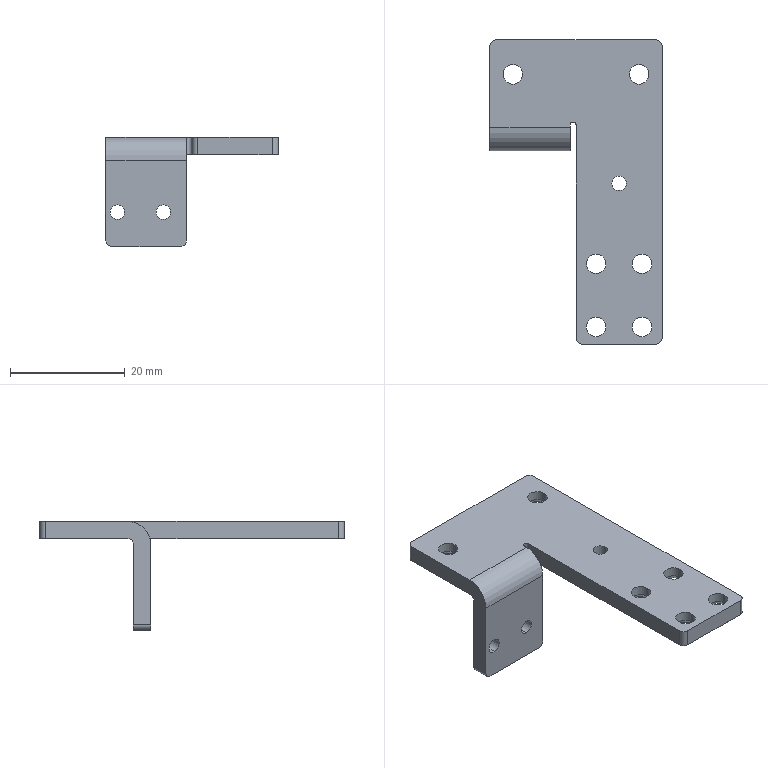Part | NX | features BREP 1 | 1 solid | 50 faces | box 30 x 53 x 19 mm | volume 3587 mm3 | cylinder 27 | cone 12 | plane 11 | commonest cylinder face diameters 3.4 x12 2 x7 2.5 x6 1 x1 8 x1